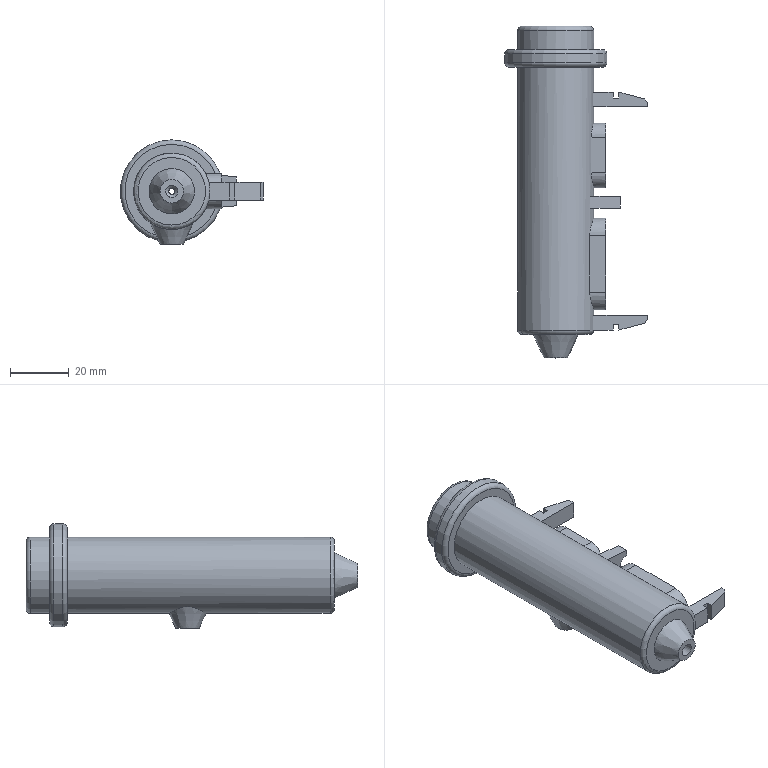Part | NX | features EXTRUDE 29, DATUM_CSYS 24, SKETCH 23, BLEND 5, CHAMFER 5, SYMBOLIC_THREAD 3, DRAFT 2 | 2 solids | 93 faces | box 48.659 x 113 x 35.5 mm | volume 22611 mm3 | plane 50 | cylinder 26 | cone 9 | torus 8 | commonest cylinder face diameters 3 x9 6 x3 2 x2 4.2 x2 7 x2 10 x2